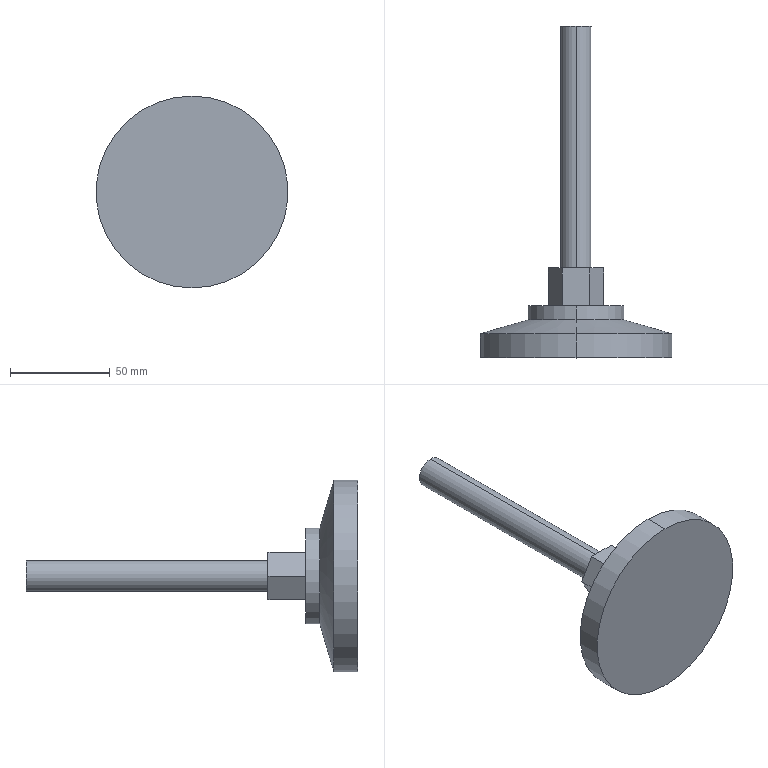Part | STEP file | large foot pad | 1 solid | 18 faces | box 96 x 166 x 96 mm | volume 161391 mm3 | plane 10 | cylinder 6 | cone 2 | commonest cylinder face diameters 15.5 x2 48 x2 96 x2
STEP:
#1=CARTESIAN_POINT('',(0.,0.,0.));
#2=DIRECTION('',(0.,0.,1.));
#3=DIRECTION('',(1.,0.,0.));
#4=AXIS2_PLACEMENT_3D('',#1,#2,#3);
#5=CARTESIAN_POINT('',(0.,12.,-48.));
#6=VERTEX_POINT('',#5);
#7=CARTESIAN_POINT('',(0.,12.,48.));
#8=VERTEX_POINT('',#7);
#9=CARTESIAN_POINT('',(0.,12.,0.));
#10=DIRECTION('',(0.,-1.,0.));
#11=DIRECTION('',(0.,0.,-1.));
#12=AXIS2_PLACEMENT_3D('',#9,#10,#11);
#13=CIRCLE('',#12,48.);
#14=CARTESIAN_POINT('',(0.,0.,0.));
#15=DIRECTION('',(0.,-1.,0.));
#16=DIRECTION('',(0.,0.,-1.));
#17=AXIS2_PLACEMENT_3D('',#14,#15,#16);
#18=CYLINDRICAL_SURFACE('',#17,48.);
#19=CARTESIAN_POINT('',(0.,-12.));
#20=DIRECTION('',(1.,0.));
#21=VECTOR('',#20,1.);
#22=LINE('',#19,#21);
#23=(GEOMETRIC_REPRESENTATION_CONTEXT(2)PARAMETRIC_REPRESENTATION_CONTEXT()REPRESENTATION_CONTEXT('',''));
#24=DEFINITIONAL_REPRESENTATION('',(#22),#23);
#25=PCURVE('',#18,#24);
#26=CARTESIAN_POINT('',(0.,12.,0.));
#27=DIRECTION('',(0.,-1.,0.));
#28=DIRECTION('',(0.,0.,-1.));
#29=AXIS2_PLACEMENT_3D('',#26,#27,#28);
#30=CONICAL_SURFACE('',#29,48.,1.287);
#31=CARTESIAN_POINT('',(0.,0.));
#32=DIRECTION('',(1.,0.));
#33=VECTOR('',#32,1.);
#34=LINE('',#31,#33);
#35=(GEOMETRIC_REPRESENTATION_CONTEXT(2)PARAMETRIC_REPRESENTATION_CONTEXT()REPRESENTATION_CONTEXT('',''));
#36=DEFINITIONAL_REPRESENTATION('',(#34),#35);
#37=PCURVE('',#30,#36);
#38=SURFACE_CURVE('',#13,(#25,#37),.PCURVE_S1.);
#39=EDGE_CURVE('',#6,#8,#38,.T.);
#40=ORIENTED_EDGE('',*,*,#39,.T.);
#41=CARTESIAN_POINT('',(0.,0.,48.));
#42=VERTEX_POINT('',#41);
#43=CARTESIAN_POINT('',(0.,0.,48.));
#44=DIRECTION('',(0.,-1.,0.));
#45=VECTOR('',#44,1.);
#46=LINE('',#43,#45);
#47=CARTESIAN_POINT('',(3.142,0.));
#48=DIRECTION('',(0.,1.));
#49=VECTOR('',#48,1.);
#50=LINE('',#47,#49);
#51=(GEOMETRIC_REPRESENTATION_CONTEXT(2)PARAMETRIC_REPRESENTATION_CONTEXT()REPRESENTATION_CONTEXT('',''));
#52=DEFINITIONAL_REPRESENTATION('',(#50),#51);
#53=PCURVE('',#18,#52);
#54=CARTESIAN_POINT('',(0.,0.,0.));
#55=DIRECTION('',(0.,-1.,0.));
#56=DIRECTION('',(0.,0.,-1.));
#57=AXIS2_PLACEMENT_3D('',#54,#55,#56);
#58=CYLINDRICAL_SURFACE('',#57,48.);
#59=CARTESIAN_POINT('',(3.142,0.));
#60=DIRECTION('',(0.,1.));
#61=VECTOR('',#60,1.);
#62=LINE('',#59,#61);
#63=(GEOMETRIC_REPRESENTATION_CONTEXT(2)PARAMETRIC_REPRESENTATION_CONTEXT()REPRESENTATION_CONTEXT('',''));
#64=DEFINITIONAL_REPRESENTATION('',(#62),#63);
#65=PCURVE('',#58,#64);
#66=SURFACE_CURVE('',#46,(#53,#65),.PCURVE_S1.);
#67=EDGE_CURVE('',#8,#42,#66,.T.);
#68=ORIENTED_EDGE('',*,*,#67,.T.);
#69=CARTESIAN_POINT('',(0.,0.,-48.));
#70=VERTEX_POINT('',#69);
#71=CARTESIAN_POINT('',(0.,0.,0.));
#72=DIRECTION('',(0.,-1.,0.));
#73=DIRECTION('',(0.,0.,-1.));
#74=AXIS2_PLACEMENT_3D('',#71,#72,#73);
#75=CIRCLE('',#74,48.);
#76=CARTESIAN_POINT('',(0.,0.));
#77=DIRECTION('',(1.,0.));
#78=VECTOR('',#77,1.);
#79=LINE('',#76,#78);
#80=(GEOMETRIC_REPRESENTATION_CONTEXT(2)PARAMETRIC_REPRESENTATION_CONTEXT()REPRESENTATION_CONTEXT('',''));
#81=DEFINITIONAL_REPRESENTATION('',(#79),#80);
#82=PCURVE('',#18,#81);
#83=CARTESIAN_POINT('',(48.,0.,0.));
#84=DIRECTION('',(0.,-1.,0.));
#85=DIRECTION('',(0.,0.,-1.));
#86=AXIS2_PLACEMENT_3D('',#83,#84,#85);
#87=PLANE('',#86);
#88=CARTESIAN_POINT('',(0.,-48.));
#89=DIRECTION('',(1.,0.));
#90=AXIS2_PLACEMENT_2D('',#88,#89);
#91=CIRCLE('',#90,48.);
#92=(GEOMETRIC_REPRESENTATION_CONTEXT(2)PARAMETRIC_REPRESENTATION_CONTEXT()REPRESENTATION_CONTEXT('',''));
#93=DEFINITIONAL_REPRESENTATION('',(#91),#92);
#94=PCURVE('',#87,#93);
#95=SURFACE_CURVE('',#75,(#82,#94),.PCURVE_S1.);
#96=EDGE_CURVE('',#70,#42,#95,.T.);
#97=ORIENTED_EDGE('',*,*,#96,.F.);
#98=CARTESIAN_POINT('',(0.,0.,-48.));
#99=DIRECTION('',(0.,-1.,0.));
#100=VECTOR('',#99,1.);
#101=LINE('',#98,#100);
#102=CARTESIAN_POINT('',(0.,0.));
#103=DIRECTION('',(0.,1.));
#104=VECTOR('',#103,1.);
#105=LINE('',#102,#104);
#106=(GEOMETRIC_REPRESENTATION_CONTEXT(2)PARAMETRIC_REPRESENTATION_CONTEXT()REPRESENTATION_CONTEXT('',''));
#107=DEFINITIONAL_REPRESENTATION('',(#105),#106);
#108=PCURVE('',#18,#107);
#109=CARTESIAN_POINT('',(6.283,0.));
#110=DIRECTION('',(0.,1.));
#111=VECTOR('',#110,1.);
#112=LINE('',#109,#111);
#113=(GEOMETRIC_REPRESENTATION_CONTEXT(2)PARAMETRIC_REPRESENTATION_CONTEXT()REPRESENTATION_CONTEXT('',''));
#114=DEFINITIONAL_REPRESENTATION('',(#112),#113);
#115=PCURVE('',#58,#114);
#116=SURFACE_CURVE('',#101,(#108,#115),.PCURVE_S1.);
#117=EDGE_CURVE('',#6,#70,#116,.T.);
#118=ORIENTED_EDGE('',*,*,#117,.F.);
#119=EDGE_LOOP('',(#40,#68,#97,#118));
#120=FACE_BOUND('',#119,.T.);
#121=ADVANCED_FACE('',(#120),#18,.T.);
#122=CARTESIAN_POINT('',(0.,19.,-24.));
#123=VERTEX_POINT('',#122);
#124=CARTESIAN_POINT('',(0.,19.,24.));
#125=VERTEX_POINT('',#124);
#126=CARTESIAN_POINT('',(0.,19.,0.));
#127=DIRECTION('',(0.,-1.,0.));
#128=DIRECTION('',(0.,0.,-1.));
#129=AXIS2_PLACEMENT_3D('',#126,#127,#128);
#130=CIRCLE('',#129,24.);
#131=CARTESIAN_POINT('',(0.,-7.));
#132=DIRECTION('',(1.,0.));
#133=VECTOR('',#132,1.);
#134=LINE('',#131,#133);
#135=(GEOMETRIC_REPRESENTATION_CONTEXT(2)PARAMETRIC_REPRESENTATION_CONTEXT()REPRESENTATION_CONTEXT('',''));
#136=DEFINITIONAL_REPRESENTATION('',(#134),#135);
#137=PCURVE('',#30,#136);
#138=CARTESIAN_POINT('',(0.,0.,0.));
#139=DIRECTION('',(0.,-1.,0.));
#140=DIRECTION('',(0.,0.,-1.));
#141=AXIS2_PLACEMENT_3D('',#138,#139,#140);
#142=CYLINDRICAL_SURFACE('',#141,24.);
#143=CARTESIAN_POINT('',(0.,-19.));
#144=DIRECTION('',(1.,0.));
#145=VECTOR('',#144,1.);
#146=LINE('',#143,#145);
#147=(GEOMETRIC_REPRESENTATION_CONTEXT(2)PARAMETRIC_REPRESENTATION_CONTEXT()REPRESENTATION_CONTEXT('',''));
#148=DEFINITIONAL_REPRESENTATION('',(#146),#147);
#149=PCURVE('',#142,#148);
#150=SURFACE_CURVE('',#130,(#137,#149),.PCURVE_S1.);
#151=EDGE_CURVE('',#123,#125,#150,.T.);
#152=ORIENTED_EDGE('',*,*,#151,.T.);
#153=CARTESIAN_POINT('',(0.,12.,48.));
#154=DIRECTION('',(0.,-0.28,0.96));
#155=VECTOR('',#154,1.);
#156=LINE('',#153,#155);
#157=CARTESIAN_POINT('',(3.142,0.));
#158=DIRECTION('',(0.,1.));
#159=VECTOR('',#158,1.);
#160=LINE('',#157,#159);
#161=(GEOMETRIC_REPRESENTATION_CONTEXT(2)PARAMETRIC_REPRESENTATION_CONTEXT()REPRESENTATION_CONTEXT('',''));
#162=DEFINITIONAL_REPRESENTATION('',(#160),#161);
#163=PCURVE('',#30,#162);
#164=CARTESIAN_POINT('',(0.,12.,0.));
#165=DIRECTION('',(0.,-1.,0.));
#166=DIRECTION('',(0.,0.,-1.));
#167=AXIS2_PLACEMENT_3D('',#164,#165,#166);
#168=CONICAL_SURFACE('',#167,48.,1.287);
#169=CARTESIAN_POINT('',(3.142,0.));
#170=DIRECTION('',(0.,1.));
#171=VECTOR('',#170,1.);
#172=LINE('',#169,#171);
#173=(GEOMETRIC_REPRESENTATION_CONTEXT(2)PARAMETRIC_REPRESENTATION_CONTEXT()REPRESENTATION_CONTEXT('',''));
#174=DEFINITIONAL_REPRESENTATION('',(#172),#173);
#175=PCURVE('',#168,#174);
#176=SURFACE_CURVE('',#156,(#163,#175),.PCURVE_S1.);
#177=EDGE_CURVE('',#125,#8,#176,.T.);
#178=ORIENTED_EDGE('',*,*,#177,.T.);
#179=ORIENTED_EDGE('',*,*,#39,.F.);
#180=CARTESIAN_POINT('',(0.,12.,-48.));
#181=DIRECTION('',(0.,-0.28,-0.96));
#182=VECTOR('',#181,1.);
#183=LINE('',#180,#182);
#184=CARTESIAN_POINT('',(0.,0.));
#185=DIRECTION('',(0.,1.));
#186=VECTOR('',#185,1.);
#187=LINE('',#184,#186);
#188=(GEOMETRIC_REPRESENTATION_CONTEXT(2)PARAMETRIC_REPRESENTATION_CONTEXT()REPRESENTATION_CONTEXT('',''));
#189=DEFINITIONAL_REPRESENTATION('',(#187),#188);
#190=PCURVE('',#30,#189);
#191=CARTESIAN_POINT('',(6.283,0.));
#192=DIRECTION('',(0.,1.));
#193=VECTOR('',#192,1.);
#194=LINE('',#191,#193);
#195=(GEOMETRIC_REPRESENTATION_CONTEXT(2)PARAMETRIC_REPRESENTATION_CONTEXT()REPRESENTATION_CONTEXT('',''));
#196=DEFINITIONAL_REPRESENTATION('',(#194),#195);
#197=PCURVE('',#168,#196);
#198=SURFACE_CURVE('',#183,(#190,#197),.PCURVE_S1.);
#199=EDGE_CURVE('',#123,#6,#198,.T.);
#200=ORIENTED_EDGE('',*,*,#199,.F.);
#201=EDGE_LOOP('',(#152,#178,#179,#200));
#202=FACE_BOUND('',#201,.T.);
#203=ADVANCED_FACE('',(#202),#30,.T.);
#204=CARTESIAN_POINT('',(0.,26.,-24.));
#205=VERTEX_POINT('',#204);
#206=CARTESIAN_POINT('',(0.,26.,24.));
#207=VERTEX_POINT('',#206);
#208=CARTESIAN_POINT('',(0.,26.,0.));
#209=DIRECTION('',(0.,-1.,0.));
#210=DIRECTION('',(0.,0.,-1.));
#211=AXIS2_PLACEMENT_3D('',#208,#209,#210);
#212=CIRCLE('',#211,24.);
#213=CARTESIAN_POINT('',(0.,-26.));
#214=DIRECTION('',(1.,0.));
#215=VECTOR('',#214,1.);
#216=LINE('',#213,#215);
#217=(GEOMETRIC_REPRESENTATION_CONTEXT(2)PARAMETRIC_REPRESENTATION_CONTEXT()REPRESENTATION_CONTEXT('',''));
#218=DEFINITIONAL_REPRESENTATION('',(#216),#217);
#219=PCURVE('',#142,#218);
#220=CARTESIAN_POINT('',(7.75,26.,0.));
#221=DIRECTION('',(0.,1.,0.));
#222=DIRECTION('',(0.,0.,1.));
#223=AXIS2_PLACEMENT_3D('',#220,#221,#222);
#224=PLANE('',#223);
#225=CARTESIAN_POINT('',(-24.,-7.75));
#226=CARTESIAN_POINT('',(-24.,33.819));
#227=CARTESIAN_POINT('',(12.,13.035));
#228=CARTESIAN_POINT('',(48.,-7.75));
#229=CARTESIAN_POINT('',(12.,-28.535));
#230=CARTESIAN_POINT('',(-24.,-49.319));
#231=CARTESIAN_POINT('',(-24.,-7.75));
#232=(BOUNDED_CURVE()B_SPLINE_CURVE(2,(#225,#226,#227,#228,#229,#230,#231),.UNSPECIFIED.,.T.,.F.)B_SPLINE_CURVE_WITH_KNOTS((1,2,2,2,2,1),(-2.094,0.,2.094,4.189,6.283,8.378),.UNSPECIFIED.)CURVE()GEOMETRIC_REPRESENTATION_ITEM()RATIONAL_B_SPLINE_CURVE((1.,0.5,1.,0.5,1.,0.5,1.))REPRESENTATION_ITEM(''));
#233=(GEOMETRIC_REPRESENTATION_CONTEXT(2)PARAMETRIC_REPRESENTATION_CONTEXT()REPRESENTATION_CONTEXT('',''));
#234=DEFINITIONAL_REPRESENTATION('',(#232),#233);
#235=PCURVE('',#224,#234);
#236=SURFACE_CURVE('',#212,(#219,#235),.PCURVE_S1.);
#237=EDGE_CURVE('',#205,#207,#236,.T.);
#238=ORIENTED_EDGE('',*,*,#237,.T.);
#239=CARTESIAN_POINT('',(0.,0.,24.));
#240=DIRECTION('',(0.,-1.,0.));
#241=VECTOR('',#240,1.);
#242=LINE('',#239,#241);
#243=CARTESIAN_POINT('',(3.142,0.));
#244=DIRECTION('',(0.,1.));
#245=VECTOR('',#244,1.);
#246=LINE('',#243,#245);
#247=(GEOMETRIC_REPRESENTATION_CONTEXT(2)PARAMETRIC_REPRESENTATION_CONTEXT()REPRESENTATION_CONTEXT('',''));
#248=DEFINITIONAL_REPRESENTATION('',(#246),#247);
#249=PCURVE('',#142,#248);
#250=CARTESIAN_POINT('',(0.,0.,0.));
#251=DIRECTION('',(0.,-1.,0.));
#252=DIRECTION('',(0.,0.,-1.));
#253=AXIS2_PLACEMENT_3D('',#250,#251,#252);
#254=CYLINDRICAL_SURFACE('',#253,24.);
#255=CARTESIAN_POINT('',(3.142,0.));
#256=DIRECTION('',(0.,1.));
#257=VECTOR('',#256,1.);
#258=LINE('',#255,#257);
#259=(GEOMETRIC_REPRESENTATION_CONTEXT(2)PARAMETRIC_REPRESENTATION_CONTEXT()REPRESENTATION_CONTEXT('',''));
#260=DEFINITIONAL_REPRESENTATION('',(#258),#259);
#261=PCURVE('',#254,#260);
#262=SURFACE_CURVE('',#242,(#249,#261),.PCURVE_S1.);
#263=EDGE_CURVE('',#207,#125,#262,.T.);
#264=ORIENTED_EDGE('',*,*,#263,.T.);
#265=ORIENTED_EDGE('',*,*,#151,.F.);
#266=CARTESIAN_POINT('',(0.,0.,-24.));
#267=DIRECTION('',(0.,-1.,0.));
#268=VECTOR('',#267,1.);
#269=LINE('',#266,#268);
#270=CARTESIAN_POINT('',(0.,0.));
#271=DIRECTION('',(0.,1.));
#272=VECTOR('',#271,1.);
#273=LINE('',#270,#272);
#274=(GEOMETRIC_REPRESENTATION_CONTEXT(2)PARAMETRIC_REPRESENTATION_CONTEXT()REPRESENTATION_CONTEXT('',''));
#275=DEFINITIONAL_REPRESENTATION('',(#273),#274);
#276=PCURVE('',#142,#275);
#277=CARTESIAN_POINT('',(6.283,0.));
#278=DIRECTION('',(0.,1.));
#279=VECTOR('',#278,1.);
#280=LINE('',#277,#279);
#281=(GEOMETRIC_REPRESENTATION_CONTEXT(2)PARAMETRIC_REPRESENTATION_CONTEXT()REPRESENTATION_CONTEXT('',''));
#282=DEFINITIONAL_REPRESENTATION('',(#280),#281);
#283=PCURVE('',#254,#282);
#284=SURFACE_CURVE('',#269,(#276,#283),.PCURVE_S1.);
#285=EDGE_CURVE('',#205,#123,#284,.T.);
#286=ORIENTED_EDGE('',*,*,#285,.F.);
#287=EDGE_LOOP('',(#238,#264,#265,#286));
#288=FACE_BOUND('',#287,.T.);
#289=ADVANCED_FACE('',(#288),#142,.T.);
#290=CARTESIAN_POINT('',(0.,166.,-7.75));
#291=VERTEX_POINT('',#290);
#292=CARTESIAN_POINT('',(0.,166.,7.75));
#293=VERTEX_POINT('',#292);
#294=CARTESIAN_POINT('',(0.,166.,0.));
#295=DIRECTION('',(0.,-1.,0.));
#296=DIRECTION('',(0.,0.,-1.));
#297=AXIS2_PLACEMENT_3D('',#294,#295,#296);
#298=CIRCLE('',#297,7.75);
#299=CARTESIAN_POINT('',(0.,0.,0.));
#300=DIRECTION('',(0.,-1.,0.));
#301=DIRECTION('',(0.,0.,-1.));
#302=AXIS2_PLACEMENT_3D('',#299,#300,#301);
#303=CYLINDRICAL_SURFACE('',#302,7.75);
#304=CARTESIAN_POINT('',(0.,-166.));
#305=DIRECTION('',(1.,0.));
#306=VECTOR('',#305,1.);
#307=LINE('',#304,#306);
#308=(GEOMETRIC_REPRESENTATION_CONTEXT(2)PARAMETRIC_REPRESENTATION_CONTEXT()REPRESENTATION_CONTEXT('',''));
#309=DEFINITIONAL_REPRESENTATION('',(#307),#308);
#310=PCURVE('',#303,#309);
#311=CARTESIAN_POINT('',(0.,166.,0.));
#312=DIRECTION('',(0.,1.,0.));
#313=DIRECTION('',(0.,0.,1.));
#314=AXIS2_PLACEMENT_3D('',#311,#312,#313);
#315=PLANE('',#314);
#316=CARTESIAN_POINT('',(-7.75,0.));
#317=CARTESIAN_POINT('',(-7.75,13.423));
#318=CARTESIAN_POINT('',(3.875,6.712));
#319=CARTESIAN_POINT('',(15.5,0.));
#320=CARTESIAN_POINT('',(3.875,-6.712));
#321=CARTESIAN_POINT('',(-7.75,-13.423));
#322=CARTESIAN_POINT('',(-7.75,0.));
#323=(BOUNDED_CURVE()B_SPLINE_CURVE(2,(#316,#317,#318,#319,#320,#321,#322),.UNSPECIFIED.,.T.,.F.)B_SPLINE_CURVE_WITH_KNOTS((1,2,2,2,2,1),(-2.094,0.,2.094,4.189,6.283,8.378),.UNSPECIFIED.)CURVE()GEOMETRIC_REPRESENTATION_ITEM()RATIONAL_B_SPLINE_CURVE((1.,0.5,1.,0.5,1.,0.5,1.))REPRESENTATION_ITEM(''));
#324=(GEOMETRIC_REPRESENTATION_CONTEXT(2)PARAMETRIC_REPRESENTATION_CONTEXT()REPRESENTATION_CONTEXT('',''));
#325=DEFINITIONAL_REPRESENTATION('',(#323),#324);
#326=PCURVE('',#315,#325);
#327=SURFACE_CURVE('',#298,(#310,#326),.PCURVE_S1.);
#328=EDGE_CURVE('',#291,#293,#327,.T.);
#329=ORIENTED_EDGE('',*,*,#328,.T.);
#330=CARTESIAN_POINT('',(0.,45.,7.75));
#331=VERTEX_POINT('',#330);
#332=CARTESIAN_POINT('',(0.,0.,7.75));
#333=DIRECTION('',(0.,-1.,0.));
#334=VECTOR('',#333,1.);
#335=LINE('',#332,#334);
#336=CARTESIAN_POINT('',(3.142,0.));
#337=DIRECTION('',(0.,1.));
#338=VECTOR('',#337,1.);
#339=LINE('',#336,#338);
#340=(GEOMETRIC_REPRESENTATION_CONTEXT(2)PARAMETRIC_REPRESENTATION_CONTEXT()REPRESENTATION_CONTEXT('',''));
#341=DEFINITIONAL_REPRESENTATION('',(#339),#340);
#342=PCURVE('',#303,#341);
#343=CARTESIAN_POINT('',(0.,0.,0.));
#344=DIRECTION('',(0.,-1.,0.));
#345=DIRECTION('',(0.,0.,-1.));
#346=AXIS2_PLACEMENT_3D('',#343,#344,#345);
#347=CYLINDRICAL_SURFACE('',#346,7.75);
#348=CARTESIAN_POINT('',(3.142,0.));
#349=DIRECTION('',(0.,1.));
#350=VECTOR('',#349,1.);
#351=LINE('',#348,#350);
#352=(GEOMETRIC_REPRESENTATION_CONTEXT(2)PARAMETRIC_REPRESENTATION_CONTEXT()REPRESENTATION_CONTEXT('',''));
#353=DEFINITIONAL_REPRESENTATION('',(#351),#352);
#354=PCURVE('',#347,#353);
#355=SURFACE_CURVE('',#335,(#342,#354),.PCURVE_S1.);
#356=EDGE_CURVE('',#293,#331,#355,.T.);
#357=ORIENTED_EDGE('',*,*,#356,.T.);
#358=CARTESIAN_POINT('',(0.,45.,-7.75));
#359=VERTEX_POINT('',#358);
#360=CARTESIAN_POINT('',(0.,45.,0.));
#361=DIRECTION('',(0.,-1.,0.));
#362=DIRECTION('',(0.,0.,-1.));
#363=AXIS2_PLACEMENT_3D('',#360,#361,#362);
#364=CIRCLE('',#363,7.75);
#365=CARTESIAN_POINT('',(0.,-45.));
#366=DIRECTION('',(1.,0.));
#367=VECTOR('',#366,1.);
#368=LINE('',#365,#367);
#369=(GEOMETRIC_REPRESENTATION_CONTEXT(2)PARAMETRIC_REPRESENTATION_CONTEXT()REPRESENTATION_CONTEXT('',''));
#370=DEFINITIONAL_REPRESENTATION('',(#368),#369);
#371=PCURVE('',#303,#370);
#372=CARTESIAN_POINT('',(0.,45.,0.));
#373=DIRECTION('',(0.,1.,0.));
#374=DIRECTION('',(0.,0.,1.));
#375=AXIS2_PLACEMENT_3D('',#372,#373,#374);
#376=PLANE('',#375);
#377=CARTESIAN_POINT('',(-7.75,0.));
#378=CARTESIAN_POINT('',(-7.75,13.423));
#379=CARTESIAN_POINT('',(3.875,6.712));
#380=CARTESIAN_POINT('',(15.5,0.));
#381=CARTESIAN_POINT('',(3.875,-6.712));
#382=CARTESIAN_POINT('',(-7.75,-13.423));
#383=CARTESIAN_POINT('',(-7.75,0.));
#384=(BOUNDED_CURVE()B_SPLINE_CURVE(2,(#377,#378,#379,#380,#381,#382,#383),.UNSPECIFIED.,.T.,.F.)B_SPLINE_CURVE_WITH_KNOTS((1,2,2,2,2,1),(-2.094,0.,2.094,4.189,6.283,8.378),.UNSPECIFIED.)CURVE()GEOMETRIC_REPRESENTATION_ITEM()RATIONAL_B_SPLINE_CURVE((1.,0.5,1.,0.5,1.,0.5,1.))REPRESENTATION_ITEM(''));
#385=(GEOMETRIC_REPRESENTATION_CONTEXT(2)PARAMETRIC_REPRESENTATION_CONTEXT()REPRESENTATION_CONTEXT('',''));
#386=DEFINITIONAL_REPRESENTATION('',(#384),#385);
#387=PCURVE('',#376,#386);
#388=SURFACE_CURVE('',#364,(#371,#387),.PCURVE_S1.);
#389=EDGE_CURVE('',#359,#331,#388,.T.);
#390=ORIENTED_EDGE('',*,*,#389,.F.);
#391=CARTESIAN_POINT('',(0.,0.,-7.75));
#392=DIRECTION('',(0.,-1.,0.));
#393=VECTOR('',#392,1.);
#394=LINE('',#391,#393);
#395=CARTESIAN_POINT('',(0.,0.));
#396=DIRECTION('',(0.,1.));
#397=VECTOR('',#396,1.);
#398=LINE('',#395,#397);
#399=(GEOMETRIC_REPRESENTATION_CONTEXT(2)PARAMETRIC_REPRESENTATION_CONTEXT()REPRESENTATION_CONTEXT('',''));
#400=DEFINITIONAL_REPRESENTATION('',(#398),#399);
#401=PCURVE('',#303,#400);
#402=CARTESIAN_POINT('',(6.283,0.));
#403=DIRECTION('',(0.,1.));
#404=VECTOR('',#403,1.);
#405=LINE('',#402,#404);
#406=(GEOMETRIC_REPRESENTATION_CONTEXT(2)PARAMETRIC_REPRESENTATION_CONTEXT()REPRESENTATION_CONTEXT('',''));
#407=DEFINITIONAL_REPRESENTATION('',(#405),#406);
#408=PCURVE('',#347,#407);
#409=SURFACE_CURVE('',#394,(#401,#408),.PCURVE_S1.);
#410=EDGE_CURVE('',#291,#359,#409,.T.);
#411=ORIENTED_EDGE('',*,*,#410,.F.);
#412=EDGE_LOOP('',(#329,#357,#390,#411));
#413=FACE_BOUND('',#412,.T.);
#414=ADVANCED_FACE('',(#413),#303,.T.);
#415=ORIENTED_EDGE('',*,*,#96,.T.);
#416=CARTESIAN_POINT('',(0.,0.,0.));
#417=DIRECTION('',(0.,-1.,0.));
#418=DIRECTION('',(0.,0.,-1.));
#419=AXIS2_PLACEMENT_3D('',#416,#417,#418);
#420=CIRCLE('',#419,48.);
#421=CARTESIAN_POINT('',(0.,-48.));
#422=DIRECTION('',(1.,0.));
#423=AXIS2_PLACEMENT_2D('',#421,#422);
#424=CIRCLE('',#423,48.);
#425=(GEOMETRIC_REPRESENTATION_CONTEXT(2)PARAMETRIC_REPRESENTATION_CONTEXT()REPRESENTATION_CONTEXT('',''));
#426=DEFINITIONAL_REPRESENTATION('',(#424),#425);
#427=PCURVE('',#87,#426);
#428=CARTESIAN_POINT('',(0.,0.));
#429=DIRECTION('',(1.,0.));
#430=VECTOR('',#429,1.);
#431=LINE('',#428,#430);
#432=(GEOMETRIC_REPRESENTATION_CONTEXT(2)PARAMETRIC_REPRESENTATION_CONTEXT()REPRESENTATION_CONTEXT('',''));
#433=DEFINITIONAL_REPRESENTATION('',(#431),#432);
#434=PCURVE('',#58,#433);
#435=SURFACE_CURVE('',#420,(#427,#434),.PCURVE_S1.);
#436=EDGE_CURVE('',#42,#70,#435,.T.);
#437=ORIENTED_EDGE('',*,*,#436,.T.);
#438=EDGE_LOOP('',(#415,#437));
#439=FACE_BOUND('',#438,.T.);
#440=ADVANCED_FACE('',(#439),#87,.T.);
#441=ORIENTED_EDGE('',*,*,#67,.F.);
#442=CARTESIAN_POINT('',(0.,12.,0.));
#443=DIRECTION('',(0.,-1.,0.));
#444=DIRECTION('',(0.,0.,-1.));
#445=AXIS2_PLACEMENT_3D('',#442,#443,#444);
#446=CIRCLE('',#445,48.);
#447=CARTESIAN_POINT('',(0.,-12.));
#448=DIRECTION('',(1.,0.));
#449=VECTOR('',#448,1.);
#450=LINE('',#447,#449);
#451=(GEOMETRIC_REPRESENTATION_CONTEXT(2)PARAMETRIC_REPRESENTATION_CONTEXT()REPRESENTATION_CONTEXT('',''));
#452=DEFINITIONAL_REPRESENTATION('',(#450),#451);
#453=PCURVE('',#58,#452);
#454=CARTESIAN_POINT('',(0.,0.));
#455=DIRECTION('',(1.,0.));
#456=VECTOR('',#455,1.);
#457=LINE('',#454,#456);
#458=(GEOMETRIC_REPRESENTATION_CONTEXT(2)PARAMETRIC_REPRESENTATION_CONTEXT()REPRESENTATION_CONTEXT('',''));
#459=DEFINITIONAL_REPRESENTATION('',(#457),#458);
#460=PCURVE('',#168,#459);
#461=SURFACE_CURVE('',#446,(#453,#460),.PCURVE_S1.);
#462=EDGE_CURVE('',#8,#6,#461,.T.);
#463=ORIENTED_EDGE('',*,*,#462,.T.);
#464=ORIENTED_EDGE('',*,*,#117,.T.);
#465=ORIENTED_EDGE('',*,*,#436,.F.);
#466=EDGE_LOOP('',(#441,#463,#464,#465));
#467=FACE_BOUND('',#466,.T.);
#468=ADVANCED_FACE('',(#467),#58,.T.);
#469=ORIENTED_EDGE('',*,*,#177,.F.);
#470=CARTESIAN_POINT('',(0.,19.,0.));
#471=DIRECTION('',(0.,-1.,0.));
#472=DIRECTION('',(0.,0.,-1.));
#473=AXIS2_PLACEMENT_3D('',#470,#471,#472);
#474=CIRCLE('',#473,24.);
#475=CARTESIAN_POINT('',(0.,-7.));
#476=DIRECTION('',(1.,0.));
#477=VECTOR('',#476,1.);
#478=LINE('',#475,#477);
#479=(GEOMETRIC_REPRESENTATION_CONTEXT(2)PARAMETRIC_REPRESENTATION_CONTEXT()REPRESENTATION_CONTEXT('',''));
#480=DEFINITIONAL_REPRESENTATION('',(#478),#479);
#481=PCURVE('',#168,#480);
#482=CARTESIAN_POINT('',(0.,-19.));
#483=DIRECTION('',(1.,0.));
#484=VECTOR('',#483,1.);
#485=LINE('',#482,#484);
#486=(GEOMETRIC_REPRESENTATION_CONTEXT(2)PARAMETRIC_REPRESENTATION_CONTEXT()REPRESENTATION_CONTEXT('',''));
#487=DEFINITIONAL_REPRESENTATION('',(#485),#486);
#488=PCURVE('',#254,#487);
#489=SURFACE_CURVE('',#474,(#481,#488),.PCURVE_S1.);
#490=EDGE_CURVE('',#125,#123,#489,.T.);
#491=ORIENTED_EDGE('',*,*,#490,.T.);
#492=ORIENTED_EDGE('',*,*,#199,.T.);
#493=ORIENTED_EDGE('',*,*,#462,.F.);
#494=EDGE_LOOP('',(#469,#491,#492,#493));
#495=FACE_BOUND('',#494,.T.);
#496=ADVANCED_FACE('',(#495),#168,.T.);
#497=ORIENTED_EDGE('',*,*,#263,.F.);
#498=CARTESIAN_POINT('',(0.,26.,0.));
#499=DIRECTION('',(0.,-1.,0.));
#500=DIRECTION('',(0.,0.,-1.));
#501=AXIS2_PLACEMENT_3D('',#498,#499,#500);
#502=CIRCLE('',#501,24.);
#503=CARTESIAN_POINT('',(0.,-26.));
#504=DIRECTION('',(1.,0.));
#505=VECTOR('',#504,1.);
#506=LINE('',#503,#505);
#507=(GEOMETRIC_REPRESENTATION_CONTEXT(2)PARAMETRIC_REPRESENTATION_CONTEXT()REPRESENTATION_CONTEXT('',''));
#508=DEFINITIONAL_REPRESENTATION('',(#506),#507);
#509=PCURVE('',#254,#508);
#510=CARTESIAN_POINT('',(-24.,-7.75));
#511=CARTESIAN_POINT('',(-24.,33.819));
#512=CARTESIAN_POINT('',(12.,13.035));
#513=CARTESIAN_POINT('',(48.,-7.75));
#514=CARTESIAN_POINT('',(12.,-28.535));
#515=CARTESIAN_POINT('',(-24.,-49.319));
#516=CARTESIAN_POINT('',(-24.,-7.75));
#517=(BOUNDED_CURVE()B_SPLINE_CURVE(2,(#510,#511,#512,#513,#514,#515,#516),.UNSPECIFIED.,.T.,.F.)B_SPLINE_CURVE_WITH_KNOTS((1,2,2,2,2,1),(-2.094,0.,2.094,4.189,6.283,8.378),.UNSPECIFIED.)CURVE()GEOMETRIC_REPRESENTATION_ITEM()RATIONAL_B_SPLINE_CURVE((1.,0.5,1.,0.5,1.,0.5,1.))REPRESENTATION_ITEM(''));
#518=(GEOMETRIC_REPRESENTATION_CONTEXT(2)PARAMETRIC_REPRESENTATION_CONTEXT()REPRESENTATION_CONTEXT('',''));
#519=DEFINITIONAL_REPRESENTATION('',(#517),#518);
#520=PCURVE('',#224,#519);
#521=SURFACE_CURVE('',#502,(#509,#520),.PCURVE_S1.);
#522=EDGE_CURVE('',#207,#205,#521,.T.);
#523=ORIENTED_EDGE('',*,*,#522,.T.);
#524=ORIENTED_EDGE('',*,*,#285,.T.);
#525=ORIENTED_EDGE('',*,*,#490,.F.);
#526=EDGE_LOOP('',(#497,#523,#524,#525));
#527=FACE_BOUND('',#526,.T.);
#528=ADVANCED_FACE('',(#527),#254,.T.);
#529=CARTESIAN_POINT('',(-13.856,26.,0.));
#530=VERTEX_POINT('',#529);
#531=CARTESIAN_POINT('',(-6.928,26.,-12.));
#532=VERTEX_POINT('',#531);
#533=CARTESIAN_POINT('',(-13.856,26.,0.));
#534=DIRECTION('',(0.5,0.,-0.866));
#535=VECTOR('',#534,1.);
#536=LINE('',#533,#535);
#537=CARTESIAN_POINT('',(0.,-21.606));
#538=DIRECTION('',(-0.866,0.5));
#539=VECTOR('',#538,1.);
#540=LINE('',#537,#539);
#541=(GEOMETRIC_REPRESENTATION_CONTEXT(2)PARAMETRIC_REPRESENTATION_CONTEXT()REPRESENTATION_CONTEXT('',''));
#542=DEFINITIONAL_REPRESENTATION('',(#540),#541);
#543=PCURVE('',#224,#542);
#544=CARTESIAN_POINT('',(-6.928,45.,-12.));
#545=DIRECTION('',(0.866,0.,0.5));
#546=DIRECTION('',(0.5,0.,-0.866));
#547=AXIS2_PLACEMENT_3D('',#544,#545,#546);
#548=PLANE('',#547);
#549=CARTESIAN_POINT('',(-13.856,-19.));
#550=DIRECTION('',(1.,0.));
#551=VECTOR('',#550,1.);
#552=LINE('',#549,#551);
#553=(GEOMETRIC_REPRESENTATION_CONTEXT(2)PARAMETRIC_REPRESENTATION_CONTEXT()REPRESENTATION_CONTEXT('',''));
#554=DEFINITIONAL_REPRESENTATION('',(#552),#553);
#555=PCURVE('',#548,#554);
#556=SURFACE_CURVE('',#536,(#543,#555),.PCURVE_S1.);
#557=EDGE_CURVE('',#530,#532,#556,.T.);
#558=ORIENTED_EDGE('',*,*,#557,.T.);
#559=CARTESIAN_POINT('',(6.928,26.,-12.));
#560=VERTEX_POINT('',#559);
#561=CARTESIAN_POINT('',(7.75,26.,-12.));
#562=DIRECTION('',(1.,0.,0.));
#563=VECTOR('',#562,1.);
#564=LINE('',#561,#563);
#565=CARTESIAN_POINT('',(-12.,0.));
#566=DIRECTION('',(0.,1.));
#567=VECTOR('',#566,1.);
#568=LINE('',#565,#567);
#569=(GEOMETRIC_REPRESENTATION_CONTEXT(2)PARAMETRIC_REPRESENTATION_CONTEXT()REPRESENTATION_CONTEXT('',''));
#570=DEFINITIONAL_REPRESENTATION('',(#568),#569);
#571=PCURVE('',#224,#570);
#572=CARTESIAN_POINT('',(6.928,45.,-12.));
#573=DIRECTION('',(0.,0.,1.));
#574=DIRECTION('',(1.,0.,0.));
#575=AXIS2_PLACEMENT_3D('',#572,#573,#574);
#576=PLANE('',#575);
#577=CARTESIAN_POINT('',(0.8218,-19.));
#578=DIRECTION('',(1.,0.));
#579=VECTOR('',#578,1.);
#580=LINE('',#577,#579);
#581=(GEOMETRIC_REPRESENTATION_CONTEXT(2)PARAMETRIC_REPRESENTATION_CONTEXT()REPRESENTATION_CONTEXT('',''));
#582=DEFINITIONAL_REPRESENTATION('',(#580),#581);
#583=PCURVE('',#576,#582);
#584=SURFACE_CURVE('',#564,(#571,#583),.PCURVE_S1.);
#585=EDGE_CURVE('',#532,#560,#584,.T.);
#586=ORIENTED_EDGE('',*,*,#585,.T.);
#587=CARTESIAN_POINT('',(13.856,26.,0.));
#588=VERTEX_POINT('',#587);
#589=CARTESIAN_POINT('',(6.928,26.,-12.));
#590=DIRECTION('',(0.5,0.,0.866));
#591=VECTOR('',#590,1.);
#592=LINE('',#589,#591);
#593=CARTESIAN_POINT('',(-12.,-0.8218));
#594=DIRECTION('',(0.866,0.5));
#595=VECTOR('',#594,1.);
#596=LINE('',#593,#595);
#597=(GEOMETRIC_REPRESENTATION_CONTEXT(2)PARAMETRIC_REPRESENTATION_CONTEXT()REPRESENTATION_CONTEXT('',''));
#598=DEFINITIONAL_REPRESENTATION('',(#596),#597);
#599=PCURVE('',#224,#598);
#600=CARTESIAN_POINT('',(13.856,45.,0.));
#601=DIRECTION('',(-0.866,0.,0.5));
#602=DIRECTION('',(0.5,0.,0.866));
#603=AXIS2_PLACEMENT_3D('',#600,#601,#602);
#604=PLANE('',#603);
#605=CARTESIAN_POINT('',(-13.856,-19.));
#606=DIRECTION('',(1.,0.));
#607=VECTOR('',#606,1.);
#608=LINE('',#605,#607);
#609=(GEOMETRIC_REPRESENTATION_CONTEXT(2)PARAMETRIC_REPRESENTATION_CONTEXT()REPRESENTATION_CONTEXT('',''));
#610=DEFINITIONAL_REPRESENTATION('',(#608),#609);
#611=PCURVE('',#604,#610);
#612=SURFACE_CURVE('',#592,(#599,#611),.PCURVE_S1.);
#613=EDGE_CURVE('',#560,#588,#612,.T.);
#614=ORIENTED_EDGE('',*,*,#613,.T.);
#615=CARTESIAN_POINT('',(6.928,26.,12.));
#616=VERTEX_POINT('',#615);
#617=CARTESIAN_POINT('',(13.856,26.,0.));
#618=DIRECTION('',(-0.5,0.,0.866));
#619=VECTOR('',#618,1.);
#620=LINE('',#617,#619);
#621=CARTESIAN_POINT('',(0.,6.106));
#622=DIRECTION('',(0.866,-0.5));
#623=VECTOR('',#622,1.);
#624=LINE('',#621,#623);
#625=(GEOMETRIC_REPRESENTATION_CONTEXT(2)PARAMETRIC_REPRESENTATION_CONTEXT()REPRESENTATION_CONTEXT('',''));
#626=DEFINITIONAL_REPRESENTATION('',(#624),#625);
#627=PCURVE('',#224,#626);
#628=CARTESIAN_POINT('',(6.928,45.,12.));
#629=DIRECTION('',(-0.866,0.,-0.5));
#630=DIRECTION('',(-0.5,0.,0.866));
#631=AXIS2_PLACEMENT_3D('',#628,#629,#630);
#632=PLANE('',#631);
#633=CARTESIAN_POINT('',(-13.856,-19.));
#634=DIRECTION('',(1.,0.));
#635=VECTOR('',#634,1.);
#636=LINE('',#633,#635);
#637=(GEOMETRIC_REPRESENTATION_CONTEXT(2)PARAMETRIC_REPRESENTATION_CONTEXT()REPRESENTATION_CONTEXT('',''));
#638=DEFINITIONAL_REPRESENTATION('',(#636),#637);
#639=PCURVE('',#632,#638);
#640=SURFACE_CURVE('',#620,(#627,#639),.PCURVE_S1.);
#641=EDGE_CURVE('',#588,#616,#640,.T.);
#642=ORIENTED_EDGE('',*,*,#641,.T.);
#643=CARTESIAN_POINT('',(-6.928,26.,12.));
#644=VERTEX_POINT('',#643);
#645=CARTESIAN_POINT('',(7.75,26.,12.));
#646=DIRECTION('',(-1.,0.,0.));
#647=VECTOR('',#646,1.);
#648=LINE('',#645,#647);
#649=CARTESIAN_POINT('',(12.,0.));
#650=DIRECTION('',(0.,-1.));
#651=VECTOR('',#650,1.);
#652=LINE('',#649,#651);
#653=(GEOMETRIC_REPRESENTATION_CONTEXT(2)PARAMETRIC_REPRESENTATION_CONTEXT()REPRESENTATION_CONTEXT('',''));
#654=DEFINITIONAL_REPRESENTATION('',(#652),#653);
#655=PCURVE('',#224,#654);
#656=CARTESIAN_POINT('',(-6.928,45.,12.));
#657=DIRECTION('',(0.,0.,-1.));
#658=DIRECTION('',(-1.,0.,0.));
#659=AXIS2_PLACEMENT_3D('',#656,#657,#658);
#660=PLANE('',#659);
#661=CARTESIAN_POINT('',(-14.678,-19.));
#662=DIRECTION('',(1.,0.));
#663=VECTOR('',#662,1.);
#664=LINE('',#661,#663);
#665=(GEOMETRIC_REPRESENTATION_CONTEXT(2)PARAMETRIC_REPRESENTATION_CONTEXT()REPRESENTATION_CONTEXT('',''));
#666=DEFINITIONAL_REPRESENTATION('',(#664),#665);
#667=PCURVE('',#660,#666);
#668=SURFACE_CURVE('',#648,(#655,#667),.PCURVE_S1.);
#669=EDGE_CURVE('',#616,#644,#668,.T.);
#670=ORIENTED_EDGE('',*,*,#669,.T.);
#671=CARTESIAN_POINT('',(-6.928,26.,12.));
#672=DIRECTION('',(-0.5,0.,-0.866));
#673=VECTOR('',#672,1.);
#674=LINE('',#671,#673);
#675=CARTESIAN_POINT('',(12.,-14.678));
#676=DIRECTION('',(-0.866,-0.5));
#677=VECTOR('',#676,1.);
#678=LINE('',#675,#677);
#679=(GEOMETRIC_REPRESENTATION_CONTEXT(2)PARAMETRIC_REPRESENTATION_CONTEXT()REPRESENTATION_CONTEXT('',''));
#680=DEFINITIONAL_REPRESENTATION('',(#678),#679);
#681=PCURVE('',#224,#680);
#682=CARTESIAN_POINT('',(-13.856,45.,0.));
#683=DIRECTION('',(0.866,0.,-0.5));
#684=DIRECTION('',(-0.5,0.,-0.866));
#685=AXIS2_PLACEMENT_3D('',#682,#683,#684);
#686=PLANE('',#685);
#687=CARTESIAN_POINT('',(-13.856,-19.));
#688=DIRECTION('',(1.,0.));
#689=VECTOR('',#688,1.);
#690=LINE('',#687,#689);
#691=(GEOMETRIC_REPRESENTATION_CONTEXT(2)PARAMETRIC_REPRESENTATION_CONTEXT()REPRESENTATION_CONTEXT('',''));
#692=DEFINITIONAL_REPRESENTATION('',(#690),#691);
#693=PCURVE('',#686,#692);
#694=SURFACE_CURVE('',#674,(#681,#693),.PCURVE_S1.);
#695=EDGE_CURVE('',#644,#530,#694,.T.);
#696=ORIENTED_EDGE('',*,*,#695,.T.);
#697=EDGE_LOOP('',(#558,#586,#614,#642,#670,#696));
#698=FACE_BOUND('',#697,.T.);
#699=ORIENTED_EDGE('',*,*,#237,.F.);
#700=ORIENTED_EDGE('',*,*,#522,.F.);
#701=EDGE_LOOP('',(#699,#700));
#702=FACE_BOUND('',#701,.T.);
#703=ADVANCED_FACE('',(#698,#702),#224,.T.);
#704=CARTESIAN_POINT('',(-6.928,45.,-12.));
#705=VERTEX_POINT('',#704);
#706=CARTESIAN_POINT('',(-6.928,45.,-12.));
#707=DIRECTION('',(0.,-1.,0.));
#708=VECTOR('',#707,1.);
#709=LINE('',#706,#708);
#710=CARTESIAN_POINT('',(-13.856,0.));
#711=DIRECTION('',(0.,-1.));
#712=VECTOR('',#711,1.);
#713=LINE('',#710,#712);
#714=(GEOMETRIC_REPRESENTATION_CONTEXT(2)PARAMETRIC_REPRESENTATION_CONTEXT()REPRESENTATION_CONTEXT('',''));
#715=DEFINITIONAL_REPRESENTATION('',(#713),#714);
#716=PCURVE('',#576,#715);
#717=CARTESIAN_POINT('',(0.,0.));
#718=DIRECTION('',(0.,-1.));
#719=VECTOR('',#718,1.);
#720=LINE('',#717,#719);
#721=(GEOMETRIC_REPRESENTATION_CONTEXT(2)PARAMETRIC_REPRESENTATION_CONTEXT()REPRESENTATION_CONTEXT('',''));
#722=DEFINITIONAL_REPRESENTATION('',(#720),#721);
#723=PCURVE('',#548,#722);
#724=SURFACE_CURVE('',#709,(#716,#723),.PCURVE_S1.);
#725=EDGE_CURVE('',#705,#532,#724,.T.);
#726=ORIENTED_EDGE('',*,*,#725,.F.);
#727=CARTESIAN_POINT('',(6.928,45.,-12.));
#728=VERTEX_POINT('',#727);
#729=CARTESIAN_POINT('',(6.928,45.,-12.));
#730=DIRECTION('',(-1.,0.,0.));
#731=VECTOR('',#730,1.);
#732=LINE('',#729,#731);
#733=CARTESIAN_POINT('',(0.,0.));
#734=DIRECTION('',(-1.,0.));
#735=VECTOR('',#734,1.);
#736=LINE('',#733,#735);
#737=(GEOMETRIC_REPRESENTATION_CONTEXT(2)PARAMETRIC_REPRESENTATION_CONTEXT()REPRESENTATION_CONTEXT('',''));
#738=DEFINITIONAL_REPRESENTATION('',(#736),#737);
#739=PCURVE('',#576,#738);
#740=CARTESIAN_POINT('',(-12.,6.928));
#741=DIRECTION('',(0.,-1.));
#742=VECTOR('',#741,1.);
#743=LINE('',#740,#742);
#744=(GEOMETRIC_REPRESENTATION_CONTEXT(2)PARAMETRIC_REPRESENTATION_CONTEXT()REPRESENTATION_CONTEXT('',''));
#745=DEFINITIONAL_REPRESENTATION('',(#743),#744);
#746=PCURVE('',#376,#745);
#747=SURFACE_CURVE('',#732,(#739,#746),.PCURVE_S1.);
#748=EDGE_CURVE('',#728,#705,#747,.T.);
#749=ORIENTED_EDGE('',*,*,#748,.F.);
#750=CARTESIAN_POINT('',(6.928,45.,-12.));
#751=DIRECTION('',(0.,1.,0.));
#752=VECTOR('',#751,1.);
#753=LINE('',#750,#752);
#754=CARTESIAN_POINT('',(0.,0.));
#755=DIRECTION('',(0.,1.));
#756=VECTOR('',#755,1.);
#757=LINE('',#754,#756);
#758=(GEOMETRIC_REPRESENTATION_CONTEXT(2)PARAMETRIC_REPRESENTATION_CONTEXT()REPRESENTATION_CONTEXT('',''));
#759=DEFINITIONAL_REPRESENTATION('',(#757),#758);
#760=PCURVE('',#576,#759);
#761=CARTESIAN_POINT('',(-13.856,0.));
#762=DIRECTION('',(0.,1.));
#763=VECTOR('',#762,1.);
#764=LINE('',#761,#763);
#765=(GEOMETRIC_REPRESENTATION_CONTEXT(2)PARAMETRIC_REPRESENTATION_CONTEXT()REPRESENTATION_CONTEXT('',''));
#766=DEFINITIONAL_REPRESENTATION('',(#764),#765);
#767=PCURVE('',#604,#766);
#768=SURFACE_CURVE('',#753,(#760,#767),.PCURVE_S1.);
#769=EDGE_CURVE('',#560,#728,#768,.T.);
#770=ORIENTED_EDGE('',*,*,#769,.F.);
#771=ORIENTED_EDGE('',*,*,#585,.F.);
#772=EDGE_LOOP('',(#726,#749,#770,#771));
#773=FACE_BOUND('',#772,.T.);
#774=ADVANCED_FACE('',(#773),#576,.F.);
#775=CARTESIAN_POINT('',(-13.856,45.,0.));
#776=VERTEX_POINT('',#775);
#777=CARTESIAN_POINT('',(-13.856,45.,0.));
#778=DIRECTION('',(0.,-1.,0.));
#779=VECTOR('',#778,1.);
#780=LINE('',#777,#779);
#781=CARTESIAN_POINT('',(-13.856,0.));
#782=DIRECTION('',(0.,-1.));
#783=VECTOR('',#782,1.);
#784=LINE('',#781,#783);
#785=(GEOMETRIC_REPRESENTATION_CONTEXT(2)PARAMETRIC_REPRESENTATION_CONTEXT()REPRESENTATION_CONTEXT('',''));
#786=DEFINITIONAL_REPRESENTATION('',(#784),#785);
#787=PCURVE('',#548,#786);
#788=CARTESIAN_POINT('',(0.,0.));
#789=DIRECTION('',(0.,-1.));
#790=VECTOR('',#789,1.);
#791=LINE('',#788,#790);
#792=(GEOMETRIC_REPRESENTATION_CONTEXT(2)PARAMETRIC_REPRESENTATION_CONTEXT()REPRESENTATION_CONTEXT('',''));
#793=DEFINITIONAL_REPRESENTATION('',(#791),#792);
#794=PCURVE('',#686,#793);
#795=SURFACE_CURVE('',#780,(#787,#794),.PCURVE_S1.);
#796=EDGE_CURVE('',#776,#530,#795,.T.);
#797=ORIENTED_EDGE('',*,*,#796,.F.);
#798=CARTESIAN_POINT('',(-6.928,45.,-12.));
#799=DIRECTION('',(-0.5,0.,0.866));
#800=VECTOR('',#799,1.);
#801=LINE('',#798,#800);
#802=CARTESIAN_POINT('',(0.,0.));
#803=DIRECTION('',(-1.,0.));
#804=VECTOR('',#803,1.);
#805=LINE('',#802,#804);
#806=(GEOMETRIC_REPRESENTATION_CONTEXT(2)PARAMETRIC_REPRESENTATION_CONTEXT()REPRESENTATION_CONTEXT('',''));
#807=DEFINITIONAL_REPRESENTATION('',(#805),#806);
#808=PCURVE('',#548,#807);
#809=CARTESIAN_POINT('',(-12.,-6.928));
#810=DIRECTION('',(0.866,-0.5));
#811=VECTOR('',#810,1.);
#812=LINE('',#809,#811);
#813=(GEOMETRIC_REPRESENTATION_CONTEXT(2)PARAMETRIC_REPRESENTATION_CONTEXT()REPRESENTATION_CONTEXT('',''));
#814=DEFINITIONAL_REPRESENTATION('',(#812),#813);
#815=PCURVE('',#376,#814);
#816=SURFACE_CURVE('',#801,(#808,#815),.PCURVE_S1.);
#817=EDGE_CURVE('',#705,#776,#816,.T.);
#818=ORIENTED_EDGE('',*,*,#817,.F.);
#819=ORIENTED_EDGE('',*,*,#725,.T.);
#820=ORIENTED_EDGE('',*,*,#557,.F.);
#821=EDGE_LOOP('',(#797,#818,#819,#820));
#822=FACE_BOUND('',#821,.T.);
#823=ADVANCED_FACE('',(#822),#548,.F.);
#824=CARTESIAN_POINT('',(-6.928,45.,12.));
#825=VERTEX_POINT('',#824);
#826=CARTESIAN_POINT('',(-6.928,45.,12.));
#827=DIRECTION('',(0.,-1.,0.));
#828=VECTOR('',#827,1.);
#829=LINE('',#826,#828);
#830=CARTESIAN_POINT('',(-13.856,0.));
#831=DIRECTION('',(0.,-1.));
#832=VECTOR('',#831,1.);
#833=LINE('',#830,#832);
#834=(GEOMETRIC_REPRESENTATION_CONTEXT(2)PARAMETRIC_REPRESENTATION_CONTEXT()REPRESENTATION_CONTEXT('',''));
#835=DEFINITIONAL_REPRESENTATION('',(#833),#834);
#836=PCURVE('',#686,#835);
#837=CARTESIAN_POINT('',(0.,0.));
#838=DIRECTION('',(0.,-1.));
#839=VECTOR('',#838,1.);
#840=LINE('',#837,#839);
#841=(GEOMETRIC_REPRESENTATION_CONTEXT(2)PARAMETRIC_REPRESENTATION_CONTEXT()REPRESENTATION_CONTEXT('',''));
#842=DEFINITIONAL_REPRESENTATION('',(#840),#841);
#843=PCURVE('',#660,#842);
#844=SURFACE_CURVE('',#829,(#836,#843),.PCURVE_S1.);
#845=EDGE_CURVE('',#825,#644,#844,.T.);
#846=ORIENTED_EDGE('',*,*,#845,.F.);
#847=CARTESIAN_POINT('',(-13.856,45.,0.));
#848=DIRECTION('',(0.5,0.,0.866));
#849=VECTOR('',#848,1.);
#850=LINE('',#847,#849);
#851=CARTESIAN_POINT('',(0.,0.));
#852=DIRECTION('',(-1.,0.));
#853=VECTOR('',#852,1.);
#854=LINE('',#851,#853);
#855=(GEOMETRIC_REPRESENTATION_CONTEXT(2)PARAMETRIC_REPRESENTATION_CONTEXT()REPRESENTATION_CONTEXT('',''));
#856=DEFINITIONAL_REPRESENTATION('',(#854),#855);
#857=PCURVE('',#686,#856);
#858=CARTESIAN_POINT('',(0.,-13.856));
#859=DIRECTION('',(0.866,0.5));
#860=VECTOR('',#859,1.);
#861=LINE('',#858,#860);
#862=(GEOMETRIC_REPRESENTATION_CONTEXT(2)PARAMETRIC_REPRESENTATION_CONTEXT()REPRESENTATION_CONTEXT('',''));
#863=DEFINITIONAL_REPRESENTATION('',(#861),#862);
#864=PCURVE('',#376,#863);
#865=SURFACE_CURVE('',#850,(#857,#864),.PCURVE_S1.);
#866=EDGE_CURVE('',#776,#825,#865,.T.);
#867=ORIENTED_EDGE('',*,*,#866,.F.);
#868=ORIENTED_EDGE('',*,*,#796,.T.);
#869=ORIENTED_EDGE('',*,*,#695,.F.);
#870=EDGE_LOOP('',(#846,#867,#868,#869));
#871=FACE_BOUND('',#870,.T.);
#872=ADVANCED_FACE('',(#871),#686,.F.);
#873=CARTESIAN_POINT('',(6.928,45.,12.));
#874=VERTEX_POINT('',#873);
#875=CARTESIAN_POINT('',(6.928,45.,12.));
#876=DIRECTION('',(0.,-1.,0.));
#877=VECTOR('',#876,1.);
#878=LINE('',#875,#877);
#879=CARTESIAN_POINT('',(-13.856,0.));
#880=DIRECTION('',(0.,-1.));
#881=VECTOR('',#880,1.);
#882=LINE('',#879,#881);
#883=(GEOMETRIC_REPRESENTATION_CONTEXT(2)PARAMETRIC_REPRESENTATION_CONTEXT()REPRESENTATION_CONTEXT('',''));
#884=DEFINITIONAL_REPRESENTATION('',(#882),#883);
#885=PCURVE('',#660,#884);
#886=CARTESIAN_POINT('',(0.,0.));
#887=DIRECTION('',(0.,-1.));
#888=VECTOR('',#887,1.);
#889=LINE('',#886,#888);
#890=(GEOMETRIC_REPRESENTATION_CONTEXT(2)PARAMETRIC_REPRESENTATION_CONTEXT()REPRESENTATION_CONTEXT('',''));
#891=DEFINITIONAL_REPRESENTATION('',(#889),#890);
#892=PCURVE('',#632,#891);
#893=SURFACE_CURVE('',#878,(#885,#892),.PCURVE_S1.);
#894=EDGE_CURVE('',#874,#616,#893,.T.);
#895=ORIENTED_EDGE('',*,*,#894,.F.);
#896=CARTESIAN_POINT('',(-6.928,45.,12.));
#897=DIRECTION('',(1.,0.,0.));
#898=VECTOR('',#897,1.);
#899=LINE('',#896,#898);
#900=CARTESIAN_POINT('',(0.,0.));
#901=DIRECTION('',(-1.,0.));
#902=VECTOR('',#901,1.);
#903=LINE('',#900,#902);
#904=(GEOMETRIC_REPRESENTATION_CONTEXT(2)PARAMETRIC_REPRESENTATION_CONTEXT()REPRESENTATION_CONTEXT('',''));
#905=DEFINITIONAL_REPRESENTATION('',(#903),#904);
#906=PCURVE('',#660,#905);
#907=CARTESIAN_POINT('',(12.,-6.928));
#908=DIRECTION('',(0.,1.));
#909=VECTOR('',#908,1.);
#910=LINE('',#907,#909);
#911=(GEOMETRIC_REPRESENTATION_CONTEXT(2)PARAMETRIC_REPRESENTATION_CONTEXT()REPRESENTATION_CONTEXT('',''));
#912=DEFINITIONAL_REPRESENTATION('',(#910),#911);
#913=PCURVE('',#376,#912);
#914=SURFACE_CURVE('',#899,(#906,#913),.PCURVE_S1.);
#915=EDGE_CURVE('',#825,#874,#914,.T.);
#916=ORIENTED_EDGE('',*,*,#915,.F.);
#917=ORIENTED_EDGE('',*,*,#845,.T.);
#918=ORIENTED_EDGE('',*,*,#669,.F.);
#919=EDGE_LOOP('',(#895,#916,#917,#918));
#920=FACE_BOUND('',#919,.T.);
#921=ADVANCED_FACE('',(#920),#660,.F.);
#922=CARTESIAN_POINT('',(13.856,45.,0.));
#923=VERTEX_POINT('',#922);
#924=CARTESIAN_POINT('',(13.856,45.,0.));
#925=DIRECTION('',(0.,-1.,0.));
#926=VECTOR('',#925,1.);
#927=LINE('',#924,#926);
#928=CARTESIAN_POINT('',(-13.856,0.));
#929=DIRECTION('',(0.,-1.));
#930=VECTOR('',#929,1.);
#931=LINE('',#928,#930);
#932=(GEOMETRIC_REPRESENTATION_CONTEXT(2)PARAMETRIC_REPRESENTATION_CONTEXT()REPRESENTATION_CONTEXT('',''));
#933=DEFINITIONAL_REPRESENTATION('',(#931),#932);
#934=PCURVE('',#632,#933);
#935=CARTESIAN_POINT('',(0.,0.));
#936=DIRECTION('',(0.,-1.));
#937=VECTOR('',#936,1.);
#938=LINE('',#935,#937);
#939=(GEOMETRIC_REPRESENTATION_CONTEXT(2)PARAMETRIC_REPRESENTATION_CONTEXT()REPRESENTATION_CONTEXT('',''));
#940=DEFINITIONAL_REPRESENTATION('',(#938),#939);
#941=PCURVE('',#604,#940);
#942=SURFACE_CURVE('',#927,(#934,#941),.PCURVE_S1.);
#943=EDGE_CURVE('',#923,#588,#942,.T.);
#944=ORIENTED_EDGE('',*,*,#943,.F.);
#945=CARTESIAN_POINT('',(6.928,45.,12.));
#946=DIRECTION('',(0.5,0.,-0.866));
#947=VECTOR('',#946,1.);
#948=LINE('',#945,#947);
#949=CARTESIAN_POINT('',(0.,0.));
#950=DIRECTION('',(-1.,0.));
#951=VECTOR('',#950,1.);
#952=LINE('',#949,#951);
#953=(GEOMETRIC_REPRESENTATION_CONTEXT(2)PARAMETRIC_REPRESENTATION_CONTEXT()REPRESENTATION_CONTEXT('',''));
#954=DEFINITIONAL_REPRESENTATION('',(#952),#953);
#955=PCURVE('',#632,#954);
#956=CARTESIAN_POINT('',(12.,6.928));
#957=DIRECTION('',(-0.866,0.5));
#958=VECTOR('',#957,1.);
#959=LINE('',#956,#958);
#960=(GEOMETRIC_REPRESENTATION_CONTEXT(2)PARAMETRIC_REPRESENTATION_CONTEXT()REPRESENTATION_CONTEXT('',''));
#961=DEFINITIONAL_REPRESENTATION('',(#959),#960);
#962=PCURVE('',#376,#961);
#963=SURFACE_CURVE('',#948,(#955,#962),.PCURVE_S1.);
#964=EDGE_CURVE('',#874,#923,#963,.T.);
#965=ORIENTED_EDGE('',*,*,#964,.F.);
#966=ORIENTED_EDGE('',*,*,#894,.T.);
#967=ORIENTED_EDGE('',*,*,#641,.F.);
#968=EDGE_LOOP('',(#944,#965,#966,#967));
#969=FACE_BOUND('',#968,.T.);
#970=ADVANCED_FACE('',(#969),#632,.F.);
#971=ORIENTED_EDGE('',*,*,#769,.T.);
#972=CARTESIAN_POINT('',(13.856,45.,0.));
#973=DIRECTION('',(-0.5,0.,-0.866));
#974=VECTOR('',#973,1.);
#975=LINE('',#972,#974);
#976=CARTESIAN_POINT('',(0.,0.));
#977=DIRECTION('',(-1.,0.));
#978=VECTOR('',#977,1.);
#979=LINE('',#976,#978);
#980=(GEOMETRIC_REPRESENTATION_CONTEXT(2)PARAMETRIC_REPRESENTATION_CONTEXT()REPRESENTATION_CONTEXT('',''));
#981=DEFINITIONAL_REPRESENTATION('',(#979),#980);
#982=PCURVE('',#604,#981);
#983=CARTESIAN_POINT('',(0.,13.856));
#984=DIRECTION('',(-0.866,-0.5));
#985=VECTOR('',#984,1.);
#986=LINE('',#983,#985);
#987=(GEOMETRIC_REPRESENTATION_CONTEXT(2)PARAMETRIC_REPRESENTATION_CONTEXT()REPRESENTATION_CONTEXT('',''));
#988=DEFINITIONAL_REPRESENTATION('',(#986),#987);
#989=PCURVE('',#376,#988);
#990=SURFACE_CURVE('',#975,(#982,#989),.PCURVE_S1.);
#991=EDGE_CURVE('',#923,#728,#990,.T.);
#992=ORIENTED_EDGE('',*,*,#991,.F.);
#993=ORIENTED_EDGE('',*,*,#943,.T.);
#994=ORIENTED_EDGE('',*,*,#613,.F.);
#995=EDGE_LOOP('',(#971,#992,#993,#994));
#996=FACE_BOUND('',#995,.T.);
#997=ADVANCED_FACE('',(#996),#604,.F.);
#998=ORIENTED_EDGE('',*,*,#866,.T.);
#999=ORIENTED_EDGE('',*,*,#915,.T.);
#1000=ORIENTED_EDGE('',*,*,#964,.T.);
#1001=ORIENTED_EDGE('',*,*,#991,.T.);
#1002=ORIENTED_EDGE('',*,*,#748,.T.);
#1003=ORIENTED_EDGE('',*,*,#817,.T.);
#1004=EDGE_LOOP('',(#998,#999,#1000,#1001,#1002,#1003));
#1005=FACE_BOUND('',#1004,.T.);
#1006=ORIENTED_EDGE('',*,*,#389,.T.);
#1007=CARTESIAN_POINT('',(0.,45.,0.));
#1008=DIRECTION('',(0.,-1.,0.));
#1009=DIRECTION('',(0.,0.,-1.));
#1010=AXIS2_PLACEMENT_3D('',#1007,#1008,#1009);
#1011=CIRCLE('',#1010,7.75);
#1012=CARTESIAN_POINT('',(-7.75,0.));
#1013=CARTESIAN_POINT('',(-7.75,13.423));
#1014=CARTESIAN_POINT('',(3.875,6.712));
#1015=CARTESIAN_POINT('',(15.5,0.));
#1016=CARTESIAN_POINT('',(3.875,-6.712));
#1017=CARTESIAN_POINT('',(-7.75,-13.423));
#1018=CARTESIAN_POINT('',(-7.75,0.));
#1019=(BOUNDED_CURVE()B_SPLINE_CURVE(2,(#1012,#1013,#1014,#1015,#1016,#1017,#1018),.UNSPECIFIED.,.T.,.F.)B_SPLINE_CURVE_WITH_KNOTS((1,2,2,2,2,1),(-2.094,0.,2.094,4.189,6.283,8.378),.UNSPECIFIED.)CURVE()GEOMETRIC_REPRESENTATION_ITEM()RATIONAL_B_SPLINE_CURVE((1.,0.5,1.,0.5,1.,0.5,1.))REPRESENTATION_ITEM(''));
#1020=(GEOMETRIC_REPRESENTATION_CONTEXT(2)PARAMETRIC_REPRESENTATION_CONTEXT()REPRESENTATION_CONTEXT('',''));
#1021=DEFINITIONAL_REPRESENTATION('',(#1019),#1020);
#1022=PCURVE('',#376,#1021);
#1023=CARTESIAN_POINT('',(0.,-45.));
#1024=DIRECTION('',(1.,0.));
#1025=VECTOR('',#1024,1.);
#1026=LINE('',#1023,#1025);
#1027=(GEOMETRIC_REPRESENTATION_CONTEXT(2)PARAMETRIC_REPRESENTATION_CONTEXT()REPRESENTATION_CONTEXT('',''));
#1028=DEFINITIONAL_REPRESENTATION('',(#1026),#1027);
#1029=PCURVE('',#347,#1028);
#1030=SURFACE_CURVE('',#1011,(#1022,#1029),.PCURVE_S1.);
#1031=EDGE_CURVE('',#331,#359,#1030,.T.);
#1032=ORIENTED_EDGE('',*,*,#1031,.T.);
#1033=EDGE_LOOP('',(#1006,#1032));
#1034=FACE_BOUND('',#1033,.T.);
#1035=ADVANCED_FACE('',(#1005,#1034),#376,.T.);
#1036=ORIENTED_EDGE('',*,*,#356,.F.);
#1037=CARTESIAN_POINT('',(0.,166.,0.));
#1038=DIRECTION('',(0.,-1.,0.));
#1039=DIRECTION('',(0.,0.,-1.));
#1040=AXIS2_PLACEMENT_3D('',#1037,#1038,#1039);
#1041=CIRCLE('',#1040,7.75);
#1042=CARTESIAN_POINT('',(0.,-166.));
#1043=DIRECTION('',(1.,0.));
#1044=VECTOR('',#1043,1.);
#1045=LINE('',#1042,#1044);
#1046=(GEOMETRIC_REPRESENTATION_CONTEXT(2)PARAMETRIC_REPRESENTATION_CONTEXT()REPRESENTATION_CONTEXT('',''));
#1047=DEFINITIONAL_REPRESENTATION('',(#1045),#1046);
#1048=PCURVE('',#347,#1047);
#1049=CARTESIAN_POINT('',(-7.75,0.));
#1050=CARTESIAN_POINT('',(-7.75,13.423));
#1051=CARTESIAN_POINT('',(3.875,6.712));
#1052=CARTESIAN_POINT('',(15.5,0.));
#1053=CARTESIAN_POINT('',(3.875,-6.712));
#1054=CARTESIAN_POINT('',(-7.75,-13.423));
#1055=CARTESIAN_POINT('',(-7.75,0.));
#1056=(BOUNDED_CURVE()B_SPLINE_CURVE(2,(#1049,#1050,#1051,#1052,#1053,#1054,#1055),.UNSPECIFIED.,.T.,.F.)B_SPLINE_CURVE_WITH_KNOTS((1,2,2,2,2,1),(-2.094,0.,2.094,4.189,6.283,8.378),.UNSPECIFIED.)CURVE()GEOMETRIC_REPRESENTATION_ITEM()RATIONAL_B_SPLINE_CURVE((1.,0.5,1.,0.5,1.,0.5,1.))REPRESENTATION_ITEM(''));
#1057=(GEOMETRIC_REPRESENTATION_CONTEXT(2)PARAMETRIC_REPRESENTATION_CONTEXT()REPRESENTATION_CONTEXT('',''));
#1058=DEFINITIONAL_REPRESENTATION('',(#1056),#1057);
#1059=PCURVE('',#315,#1058);
#1060=SURFACE_CURVE('',#1041,(#1048,#1059),.PCURVE_S1.);
#1061=EDGE_CURVE('',#293,#291,#1060,.T.);
#1062=ORIENTED_EDGE('',*,*,#1061,.T.);
#1063=ORIENTED_EDGE('',*,*,#410,.T.);
#1064=ORIENTED_EDGE('',*,*,#1031,.F.);
#1065=EDGE_LOOP('',(#1036,#1062,#1063,#1064));
#1066=FACE_BOUND('',#1065,.T.);
#1067=ADVANCED_FACE('',(#1066),#347,.T.);
#1068=ORIENTED_EDGE('',*,*,#328,.F.);
#1069=ORIENTED_EDGE('',*,*,#1061,.F.);
#1070=EDGE_LOOP('',(#1068,#1069));
#1071=FACE_BOUND('',#1070,.T.);
#1072=ADVANCED_FACE('',(#1071),#315,.T.);
#1073=CLOSED_SHELL('',(#121,#203,#289,#414,#440,#468,#496,#528,#703,#774,#823,#872,#921,#970,#997,#1035,#1067,#1072));
#1074=MANIFOLD_SOLID_BREP('',#1073);
#1075=(LENGTH_UNIT()NAMED_UNIT(*)SI_UNIT(.MILLI.,.METRE.));
#1076=UNCERTAINTY_MEASURE_WITH_UNIT(LENGTH_MEASURE(0.0000001),#1075,'','');
#1077=(NAMED_UNIT(*)PLANE_ANGLE_UNIT()SI_UNIT($,.RADIAN.));
#1078=(NAMED_UNIT(*)SI_UNIT($,.STERADIAN.)SOLID_ANGLE_UNIT());
#1079=(GEOMETRIC_REPRESENTATION_CONTEXT(3)GLOBAL_UNCERTAINTY_ASSIGNED_CONTEXT((#1076))GLOBAL_UNIT_ASSIGNED_CONTEXT((#1075,#1077,#1078))REPRESENTATION_CONTEXT('',''));
#1080=ADVANCED_BREP_SHAPE_REPRESENTATION('',(#4,#1074),#1079);